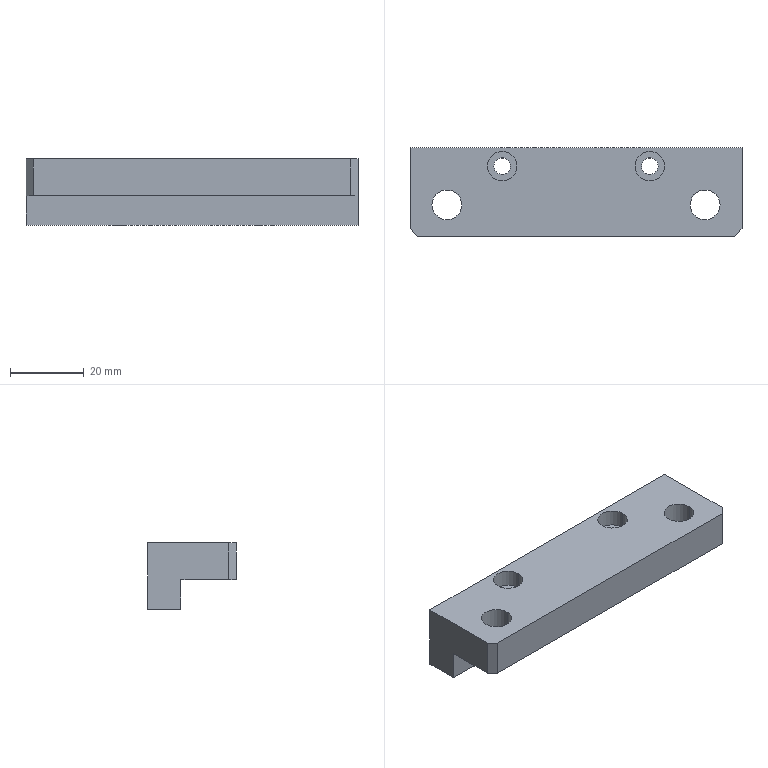Part | STEP file | 2052 Spring mounting plate A | 1 solid | 30 faces | box 90 x 24 x 18 mm | volume 25874 mm3 | cylinder 16 | plane 14 | commonest cylinder face diameters 4.5 x4 8 x4 8.1 x4 12 x4